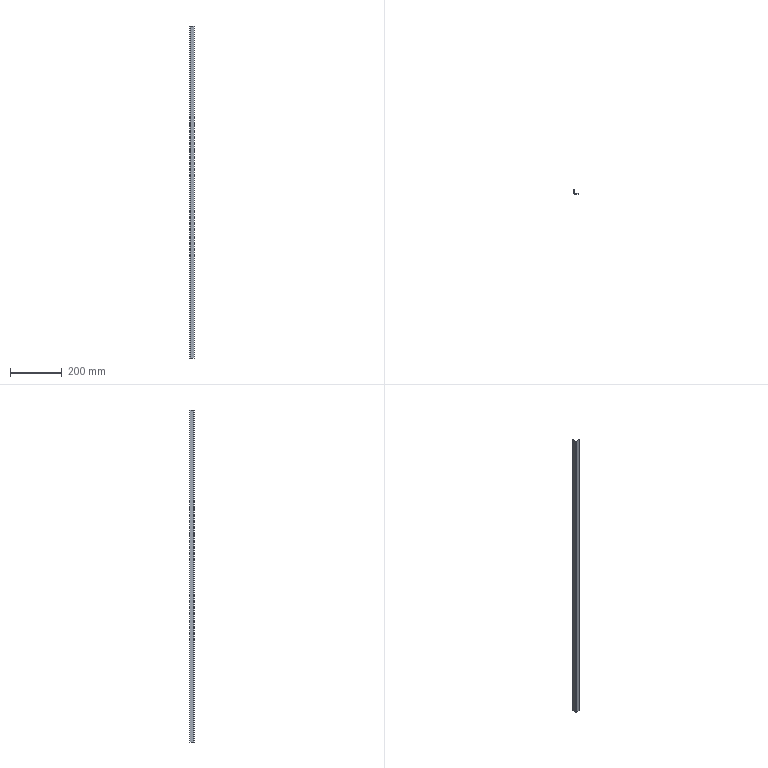Part | NX | features solid 2 | 1 solid | 10 faces | box 16.5 x 16.5 x 1285 mm | volume 58855 mm3 | plane 8 | cylinder 2 | commonest cylinder face diameters 3 x1 6 x1
STEP:
#1=CARTESIAN_POINT('',(1095.,508.5,1290.));
#2=VERTEX_POINT('',#1);
#3=CARTESIAN_POINT('',(1108.5,508.5,1290.));
#4=VERTEX_POINT('',#3);
#5=CARTESIAN_POINT('',(1093.5,508.5,1290.));
#6=DIRECTION('',(1.,0.,0.));
#7=VECTOR('',#6,1000.);
#8=LINE('',#5,#7);
#9=EDGE_CURVE('',#2,#4,#8,.T.);
#10=ORIENTED_EDGE('',*,*,#9,.T.);
#11=CARTESIAN_POINT('',(1108.5,508.5,5.));
#12=VERTEX_POINT('',#11);
#13=CARTESIAN_POINT('',(1108.5,508.5,5.));
#14=DIRECTION('',(0.,0.,1.));
#15=VECTOR('',#14,1000.);
#16=LINE('',#13,#15);
#17=EDGE_CURVE('',#12,#4,#16,.T.);
#18=ORIENTED_EDGE('',*,*,#17,.F.);
#19=CARTESIAN_POINT('',(1095.,508.5,5.));
#20=VERTEX_POINT('',#19);
#21=CARTESIAN_POINT('',(1093.5,508.5,5.));
#22=DIRECTION('',(1.,0.,0.));
#23=VECTOR('',#22,1000.);
#24=LINE('',#21,#23);
#25=EDGE_CURVE('',#20,#12,#24,.T.);
#26=ORIENTED_EDGE('',*,*,#25,.F.);
#27=CARTESIAN_POINT('',(1095.,508.5,5.));
#28=DIRECTION('',(0.,0.,1.));
#29=VECTOR('',#28,1000.);
#30=LINE('',#27,#29);
#31=EDGE_CURVE('',#20,#2,#30,.T.);
#32=ORIENTED_EDGE('',*,*,#31,.T.);
#33=EDGE_LOOP('',(#10,#18,#26,#32));
#34=FACE_BOUND('',#33,.T.);
#35=CARTESIAN_POINT('',(1093.5,508.5,5.));
#36=DIRECTION('',(0.,-1.,0.));
#37=DIRECTION('',(-1.,0.,0.));
#38=AXIS2_PLACEMENT_3D('',#35,#36,#37);
#39=PLANE('',#38);
#40=ADVANCED_FACE('',(#34),#39,.F.);
#41=CARTESIAN_POINT('',(1093.5,510.,1290.));
#42=VERTEX_POINT('',#41);
#43=CARTESIAN_POINT('',(1095.,510.,1290.));
#44=DIRECTION('',(0.,0.,1.));
#45=DIRECTION('',(0.,1.,0.));
#46=AXIS2_PLACEMENT_3D('',#43,#44,#45);
#47=CIRCLE('',#46,1.5);
#48=EDGE_CURVE('',#42,#2,#47,.T.);
#49=ORIENTED_EDGE('',*,*,#48,.T.);
#50=ORIENTED_EDGE('',*,*,#31,.F.);
#51=CARTESIAN_POINT('',(1093.5,510.,5.));
#52=VERTEX_POINT('',#51);
#53=CARTESIAN_POINT('',(1095.,510.,5.));
#54=DIRECTION('',(0.,0.,1.));
#55=DIRECTION('',(0.,1.,0.));
#56=AXIS2_PLACEMENT_3D('',#53,#54,#55);
#57=CIRCLE('',#56,1.5);
#58=EDGE_CURVE('',#52,#20,#57,.T.);
#59=ORIENTED_EDGE('',*,*,#58,.F.);
#60=CARTESIAN_POINT('',(1093.5,510.,5.));
#61=DIRECTION('',(0.,0.,1.));
#62=VECTOR('',#61,1000.);
#63=LINE('',#60,#62);
#64=EDGE_CURVE('',#52,#42,#63,.T.);
#65=ORIENTED_EDGE('',*,*,#64,.T.);
#66=EDGE_LOOP('',(#49,#50,#59,#65));
#67=FACE_BOUND('',#66,.T.);
#68=CARTESIAN_POINT('',(1095.,510.,5.));
#69=DIRECTION('',(0.,0.,1.));
#70=DIRECTION('',(0.,-1.,0.));
#71=AXIS2_PLACEMENT_3D('',#68,#69,#70);
#72=CYLINDRICAL_SURFACE('',#71,1.5);
#73=ADVANCED_FACE('',(#67),#72,.F.);
#74=CARTESIAN_POINT('',(1093.5,523.5,1290.));
#75=VERTEX_POINT('',#74);
#76=CARTESIAN_POINT('',(1093.5,523.5,1290.));
#77=DIRECTION('',(0.,-1.,0.));
#78=VECTOR('',#77,1000.);
#79=LINE('',#76,#78);
#80=EDGE_CURVE('',#75,#42,#79,.T.);
#81=ORIENTED_EDGE('',*,*,#80,.T.);
#82=ORIENTED_EDGE('',*,*,#64,.F.);
#83=CARTESIAN_POINT('',(1093.5,523.5,5.));
#84=VERTEX_POINT('',#83);
#85=CARTESIAN_POINT('',(1093.5,523.5,5.));
#86=DIRECTION('',(0.,-1.,0.));
#87=VECTOR('',#86,1000.);
#88=LINE('',#85,#87);
#89=EDGE_CURVE('',#84,#52,#88,.T.);
#90=ORIENTED_EDGE('',*,*,#89,.F.);
#91=CARTESIAN_POINT('',(1093.5,523.5,5.));
#92=DIRECTION('',(0.,0.,1.));
#93=VECTOR('',#92,1000.);
#94=LINE('',#91,#93);
#95=EDGE_CURVE('',#84,#75,#94,.T.);
#96=ORIENTED_EDGE('',*,*,#95,.T.);
#97=EDGE_LOOP('',(#81,#82,#90,#96));
#98=FACE_BOUND('',#97,.T.);
#99=CARTESIAN_POINT('',(1093.5,523.5,5.));
#100=DIRECTION('',(-1.,0.,0.));
#101=DIRECTION('',(0.,0.,1.));
#102=AXIS2_PLACEMENT_3D('',#99,#100,#101);
#103=PLANE('',#102);
#104=ADVANCED_FACE('',(#98),#103,.F.);
#105=CARTESIAN_POINT('',(1095.,507.,1290.));
#106=VERTEX_POINT('',#105);
#107=CARTESIAN_POINT('',(1108.5,507.,1290.));
#108=VERTEX_POINT('',#107);
#109=CARTESIAN_POINT('',(1093.5,507.,1290.));
#110=DIRECTION('',(1.,0.,0.));
#111=VECTOR('',#110,1000.);
#112=LINE('',#109,#111);
#113=EDGE_CURVE('',#106,#108,#112,.T.);
#114=ORIENTED_EDGE('',*,*,#113,.F.);
#115=CARTESIAN_POINT('',(1095.,507.,5.));
#116=VERTEX_POINT('',#115);
#117=CARTESIAN_POINT('',(1095.,507.,5.));
#118=DIRECTION('',(0.,0.,1.));
#119=VECTOR('',#118,1000.);
#120=LINE('',#117,#119);
#121=EDGE_CURVE('',#116,#106,#120,.T.);
#122=ORIENTED_EDGE('',*,*,#121,.F.);
#123=CARTESIAN_POINT('',(1108.5,507.,5.));
#124=VERTEX_POINT('',#123);
#125=CARTESIAN_POINT('',(1093.5,507.,5.));
#126=DIRECTION('',(1.,0.,0.));
#127=VECTOR('',#126,1000.);
#128=LINE('',#125,#127);
#129=EDGE_CURVE('',#116,#124,#128,.T.);
#130=ORIENTED_EDGE('',*,*,#129,.T.);
#131=CARTESIAN_POINT('',(1108.5,507.,5.));
#132=DIRECTION('',(0.,0.,1.));
#133=VECTOR('',#132,1000.);
#134=LINE('',#131,#133);
#135=EDGE_CURVE('',#124,#108,#134,.T.);
#136=ORIENTED_EDGE('',*,*,#135,.T.);
#137=EDGE_LOOP('',(#114,#122,#130,#136));
#138=FACE_BOUND('',#137,.T.);
#139=CARTESIAN_POINT('',(1093.5,507.,5.));
#140=DIRECTION('',(0.,-1.,0.));
#141=DIRECTION('',(-1.,0.,0.));
#142=AXIS2_PLACEMENT_3D('',#139,#140,#141);
#143=PLANE('',#142);
#144=ADVANCED_FACE('',(#138),#143,.T.);
#145=CARTESIAN_POINT('',(1092.,510.,1290.));
#146=VERTEX_POINT('',#145);
#147=CARTESIAN_POINT('',(1095.,510.,1290.));
#148=DIRECTION('',(0.,0.,1.));
#149=DIRECTION('',(0.,-1.,0.));
#150=AXIS2_PLACEMENT_3D('',#147,#148,#149);
#151=CIRCLE('',#150,3.);
#152=EDGE_CURVE('',#146,#106,#151,.T.);
#153=ORIENTED_EDGE('',*,*,#152,.F.);
#154=CARTESIAN_POINT('',(1092.,510.,5.));
#155=VERTEX_POINT('',#154);
#156=CARTESIAN_POINT('',(1092.,510.,5.));
#157=DIRECTION('',(0.,0.,1.));
#158=VECTOR('',#157,1000.);
#159=LINE('',#156,#158);
#160=EDGE_CURVE('',#155,#146,#159,.T.);
#161=ORIENTED_EDGE('',*,*,#160,.F.);
#162=CARTESIAN_POINT('',(1095.,510.,5.));
#163=DIRECTION('',(0.,0.,1.));
#164=DIRECTION('',(0.,-1.,0.));
#165=AXIS2_PLACEMENT_3D('',#162,#163,#164);
#166=CIRCLE('',#165,3.);
#167=EDGE_CURVE('',#155,#116,#166,.T.);
#168=ORIENTED_EDGE('',*,*,#167,.T.);
#169=ORIENTED_EDGE('',*,*,#121,.T.);
#170=EDGE_LOOP('',(#153,#161,#168,#169));
#171=FACE_BOUND('',#170,.T.);
#172=CARTESIAN_POINT('',(1095.,510.,5.));
#173=DIRECTION('',(0.,0.,1.));
#174=DIRECTION('',(0.,-1.,0.));
#175=AXIS2_PLACEMENT_3D('',#172,#173,#174);
#176=CYLINDRICAL_SURFACE('',#175,3.);
#177=ADVANCED_FACE('',(#171),#176,.T.);
#178=CARTESIAN_POINT('',(1092.,523.5,1290.));
#179=VERTEX_POINT('',#178);
#180=CARTESIAN_POINT('',(1092.,523.5,1290.));
#181=DIRECTION('',(0.,-1.,0.));
#182=VECTOR('',#181,1000.);
#183=LINE('',#180,#182);
#184=EDGE_CURVE('',#179,#146,#183,.T.);
#185=ORIENTED_EDGE('',*,*,#184,.F.);
#186=CARTESIAN_POINT('',(1092.,523.5,5.));
#187=VERTEX_POINT('',#186);
#188=CARTESIAN_POINT('',(1092.,523.5,5.));
#189=DIRECTION('',(0.,0.,1.));
#190=VECTOR('',#189,1000.);
#191=LINE('',#188,#190);
#192=EDGE_CURVE('',#187,#179,#191,.T.);
#193=ORIENTED_EDGE('',*,*,#192,.F.);
#194=CARTESIAN_POINT('',(1092.,523.5,5.));
#195=DIRECTION('',(0.,-1.,0.));
#196=VECTOR('',#195,1000.);
#197=LINE('',#194,#196);
#198=EDGE_CURVE('',#187,#155,#197,.T.);
#199=ORIENTED_EDGE('',*,*,#198,.T.);
#200=ORIENTED_EDGE('',*,*,#160,.T.);
#201=EDGE_LOOP('',(#185,#193,#199,#200));
#202=FACE_BOUND('',#201,.T.);
#203=CARTESIAN_POINT('',(1092.,523.5,5.));
#204=DIRECTION('',(-1.,0.,0.));
#205=DIRECTION('',(0.,0.,1.));
#206=AXIS2_PLACEMENT_3D('',#203,#204,#205);
#207=PLANE('',#206);
#208=ADVANCED_FACE('',(#202),#207,.T.);
#209=ORIENTED_EDGE('',*,*,#95,.F.);
#210=CARTESIAN_POINT('',(1093.5,523.5,5.));
#211=DIRECTION('',(-1.,0.,0.));
#212=VECTOR('',#211,1000.);
#213=LINE('',#210,#212);
#214=EDGE_CURVE('',#84,#187,#213,.T.);
#215=ORIENTED_EDGE('',*,*,#214,.T.);
#216=ORIENTED_EDGE('',*,*,#192,.T.);
#217=CARTESIAN_POINT('',(1093.5,523.5,1290.));
#218=DIRECTION('',(-1.,0.,0.));
#219=VECTOR('',#218,1000.);
#220=LINE('',#217,#219);
#221=EDGE_CURVE('',#75,#179,#220,.T.);
#222=ORIENTED_EDGE('',*,*,#221,.F.);
#223=EDGE_LOOP('',(#209,#215,#216,#222));
#224=FACE_BOUND('',#223,.T.);
#225=CARTESIAN_POINT('',(1093.5,523.5,5.));
#226=DIRECTION('',(0.,-1.,0.));
#227=DIRECTION('',(-1.,0.,0.));
#228=AXIS2_PLACEMENT_3D('',#225,#226,#227);
#229=PLANE('',#228);
#230=ADVANCED_FACE('',(#224),#229,.F.);
#231=ORIENTED_EDGE('',*,*,#184,.T.);
#232=ORIENTED_EDGE('',*,*,#152,.T.);
#233=ORIENTED_EDGE('',*,*,#113,.T.);
#234=CARTESIAN_POINT('',(1108.5,508.5,1290.));
#235=DIRECTION('',(0.,-1.,0.));
#236=VECTOR('',#235,1000.);
#237=LINE('',#234,#236);
#238=EDGE_CURVE('',#4,#108,#237,.T.);
#239=ORIENTED_EDGE('',*,*,#238,.F.);
#240=ORIENTED_EDGE('',*,*,#9,.F.);
#241=ORIENTED_EDGE('',*,*,#48,.F.);
#242=ORIENTED_EDGE('',*,*,#80,.F.);
#243=ORIENTED_EDGE('',*,*,#221,.T.);
#244=EDGE_LOOP('',(#231,#232,#233,#239,#240,#241,#242,#243));
#245=FACE_BOUND('',#244,.T.);
#246=CARTESIAN_POINT('',(1093.5,523.5,1290.));
#247=DIRECTION('',(0.,0.,-1.));
#248=DIRECTION('',(-1.,0.,0.));
#249=AXIS2_PLACEMENT_3D('',#246,#247,#248);
#250=PLANE('',#249);
#251=ADVANCED_FACE('',(#245),#250,.F.);
#252=CARTESIAN_POINT('',(1108.5,508.5,5.));
#253=DIRECTION('',(0.,-1.,0.));
#254=VECTOR('',#253,1000.);
#255=LINE('',#252,#254);
#256=EDGE_CURVE('',#12,#124,#255,.T.);
#257=ORIENTED_EDGE('',*,*,#256,.F.);
#258=ORIENTED_EDGE('',*,*,#17,.T.);
#259=ORIENTED_EDGE('',*,*,#238,.T.);
#260=ORIENTED_EDGE('',*,*,#135,.F.);
#261=EDGE_LOOP('',(#257,#258,#259,#260));
#262=FACE_BOUND('',#261,.T.);
#263=CARTESIAN_POINT('',(1108.5,508.5,5.));
#264=DIRECTION('',(1.,0.,0.));
#265=DIRECTION('',(0.,0.,-1.));
#266=AXIS2_PLACEMENT_3D('',#263,#264,#265);
#267=PLANE('',#266);
#268=ADVANCED_FACE('',(#262),#267,.T.);
#269=ORIENTED_EDGE('',*,*,#129,.F.);
#270=ORIENTED_EDGE('',*,*,#167,.F.);
#271=ORIENTED_EDGE('',*,*,#198,.F.);
#272=ORIENTED_EDGE('',*,*,#214,.F.);
#273=ORIENTED_EDGE('',*,*,#89,.T.);
#274=ORIENTED_EDGE('',*,*,#58,.T.);
#275=ORIENTED_EDGE('',*,*,#25,.T.);
#276=ORIENTED_EDGE('',*,*,#256,.T.);
#277=EDGE_LOOP('',(#269,#270,#271,#272,#273,#274,#275,#276));
#278=FACE_BOUND('',#277,.T.);
#279=CARTESIAN_POINT('',(1093.5,508.5,5.));
#280=DIRECTION('',(0.,0.,-1.));
#281=DIRECTION('',(-1.,0.,0.));
#282=AXIS2_PLACEMENT_3D('',#279,#280,#281);
#283=PLANE('',#282);
#284=ADVANCED_FACE('',(#278),#283,.T.);
#285=CLOSED_SHELL('',(#40,#73,#104,#144,#177,#208,#230,#251,#268,#284));
#286=MANIFOLD_SOLID_BREP('',#285);
#287=(LENGTH_UNIT()NAMED_UNIT(*)SI_UNIT(.MILLI.,.METRE.));
#288=UNCERTAINTY_MEASURE_WITH_UNIT(LENGTH_MEASURE(0.00001),#287,'','');
#289=(NAMED_UNIT(*)PLANE_ANGLE_UNIT()SI_UNIT($,.RADIAN.));
#290=(NAMED_UNIT(*)SI_UNIT($,.STERADIAN.)SOLID_ANGLE_UNIT());
#291=(GEOMETRIC_REPRESENTATION_CONTEXT(3)GLOBAL_UNCERTAINTY_ASSIGNED_CONTEXT((#288))GLOBAL_UNIT_ASSIGNED_CONTEXT((#287,#289,#290))REPRESENTATION_CONTEXT('',''));
#292=ADVANCED_BREP_SHAPE_REPRESENTATION('',(#286),#291);